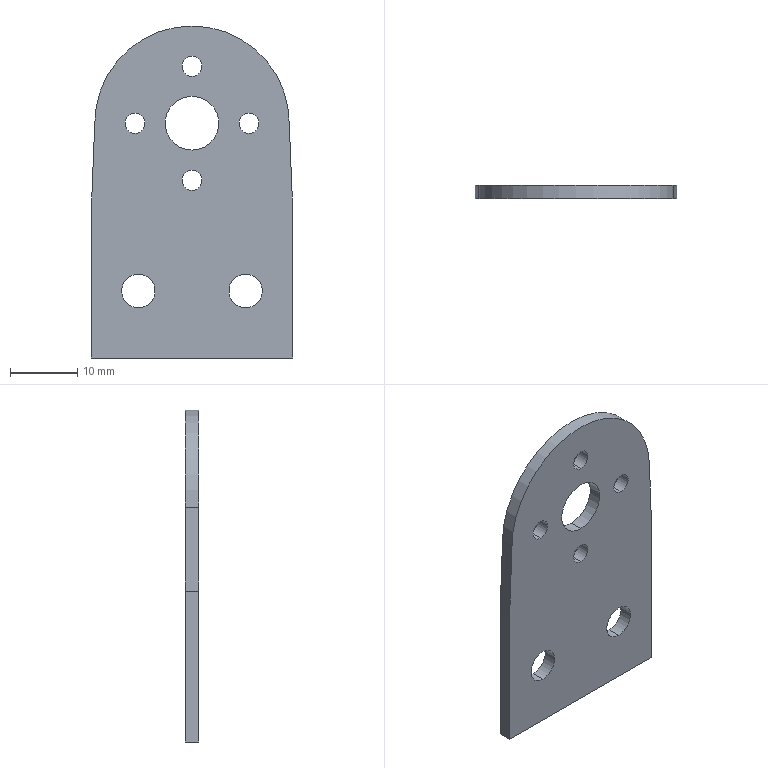Part | STEP file | Smooth shaft 370 bracket | 1 solid | 22 faces | box 30 x 2 x 49.5 mm | volume 2512 mm3 | cylinder 15 | plane 7 | commonest cylinder face diameters 3 x8 5 x4 8 x2 29 x1